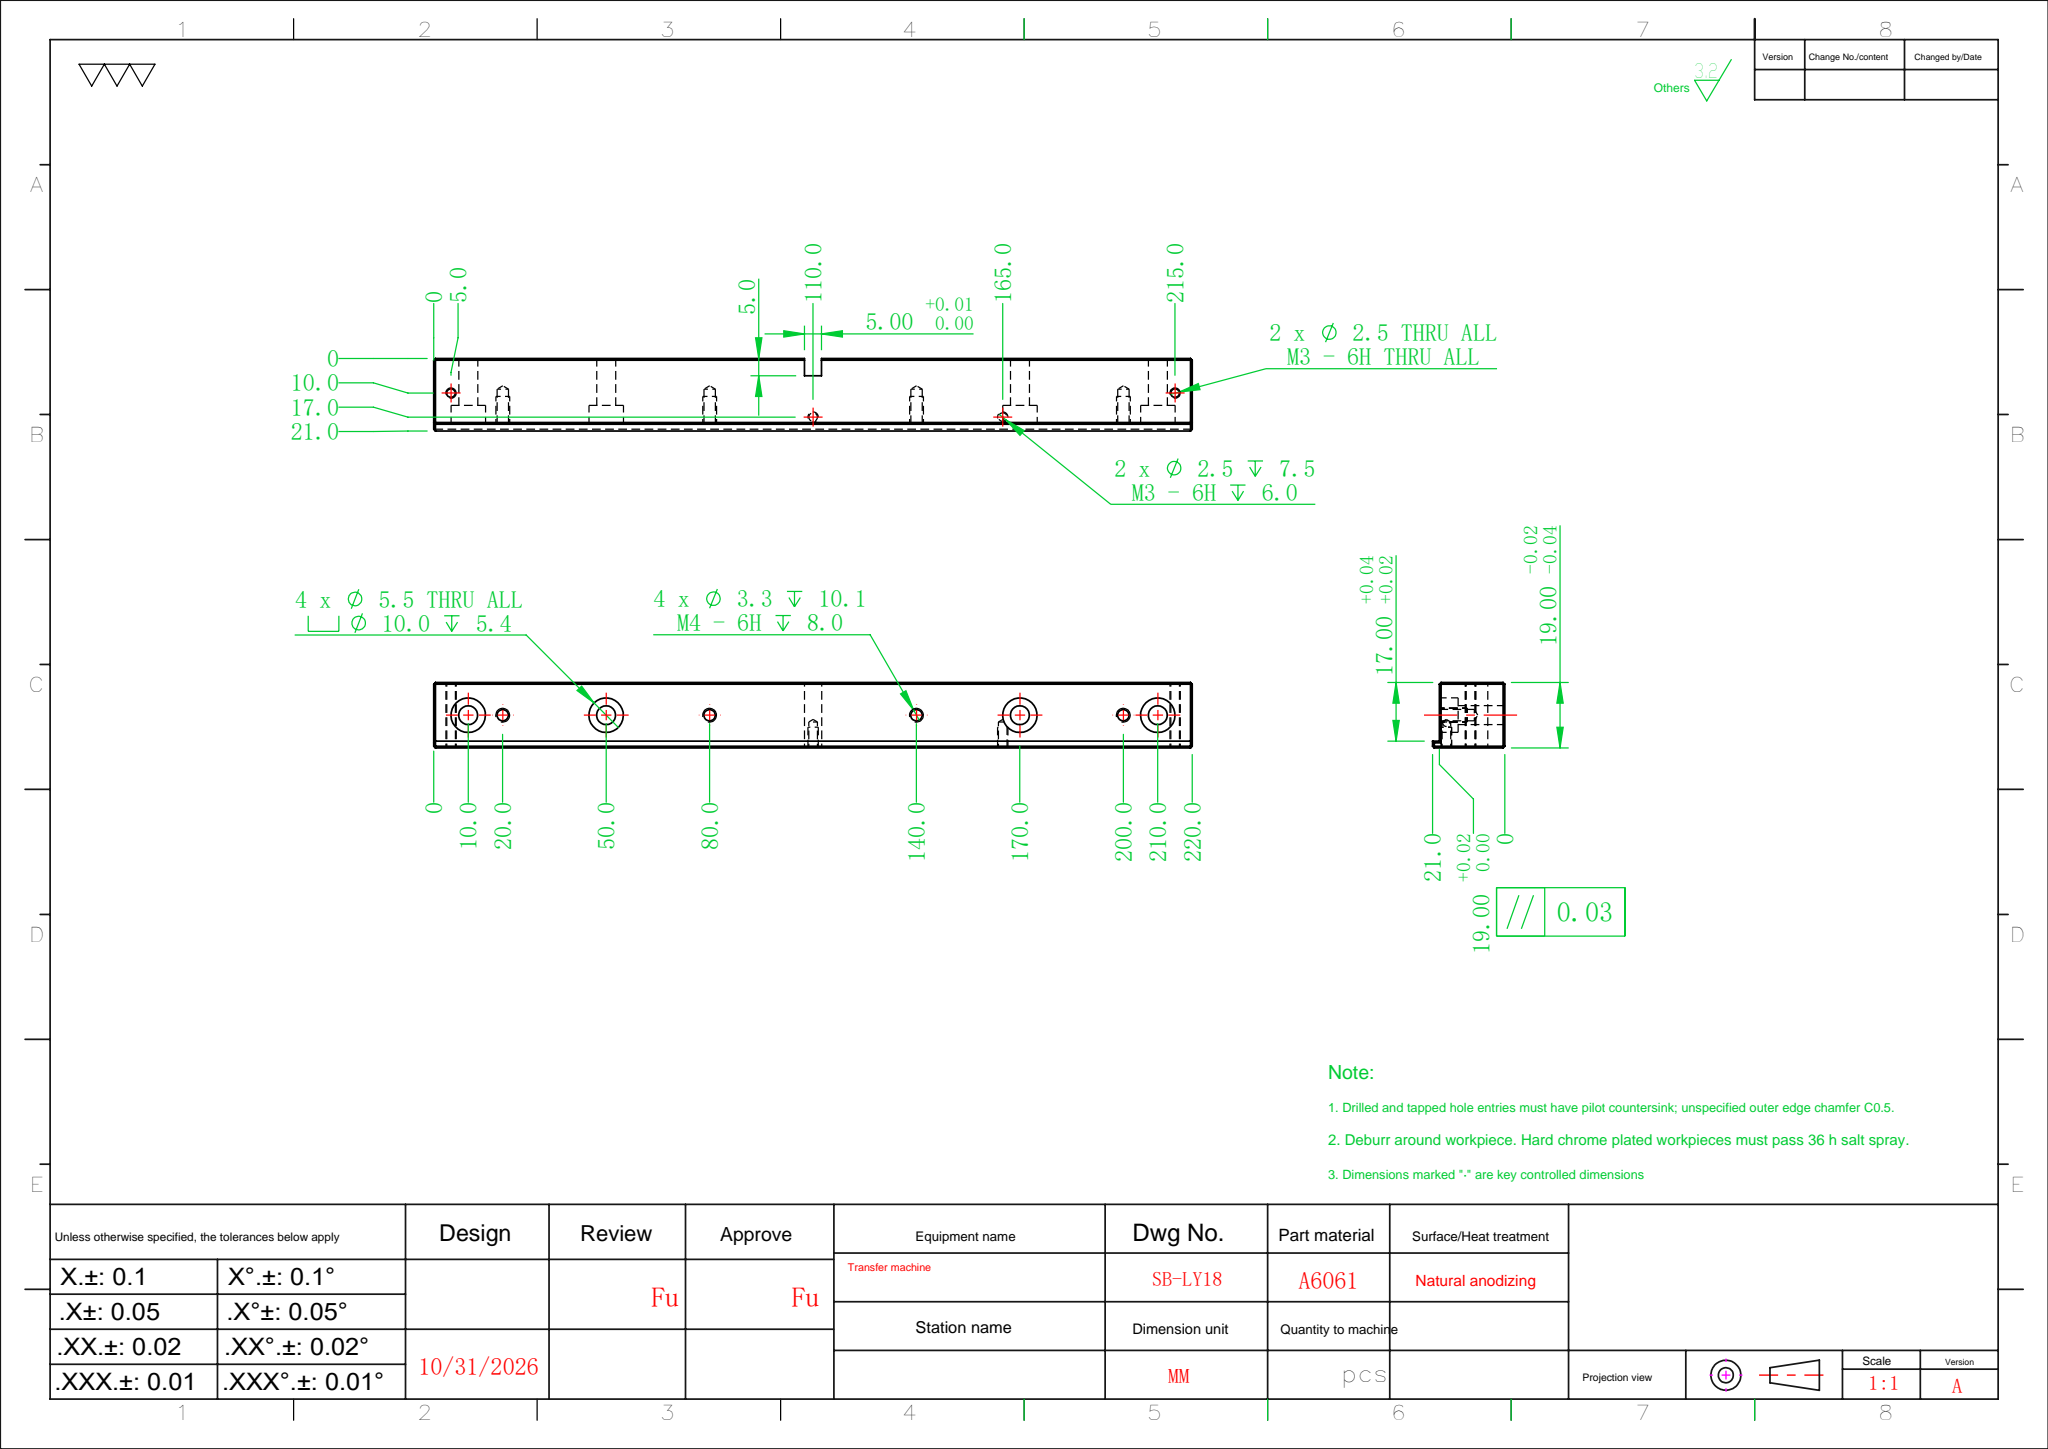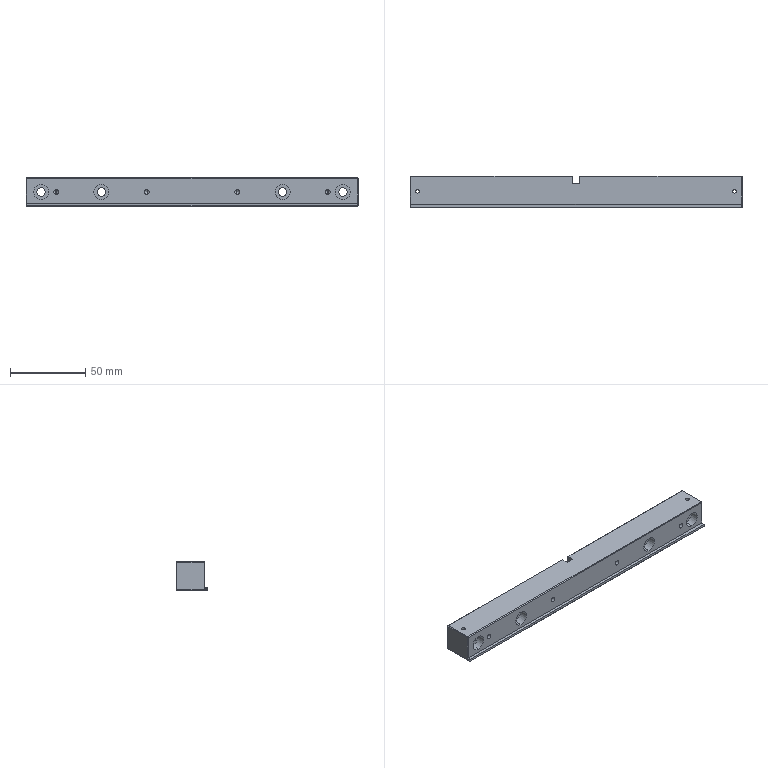Part | SolidWorks | features HoleWzd 4, ICE 2, Chamfer 1, Cut 1, Extrusion 1 | 1 solid | 86 faces | box 220 x 21 x 19 mm | volume 76090 mm3 | plane 42 | cylinder 32 | cone 12 | commonest cylinder face diameters 2.5 x8 3.3 x8 5.5 x8 10 x8